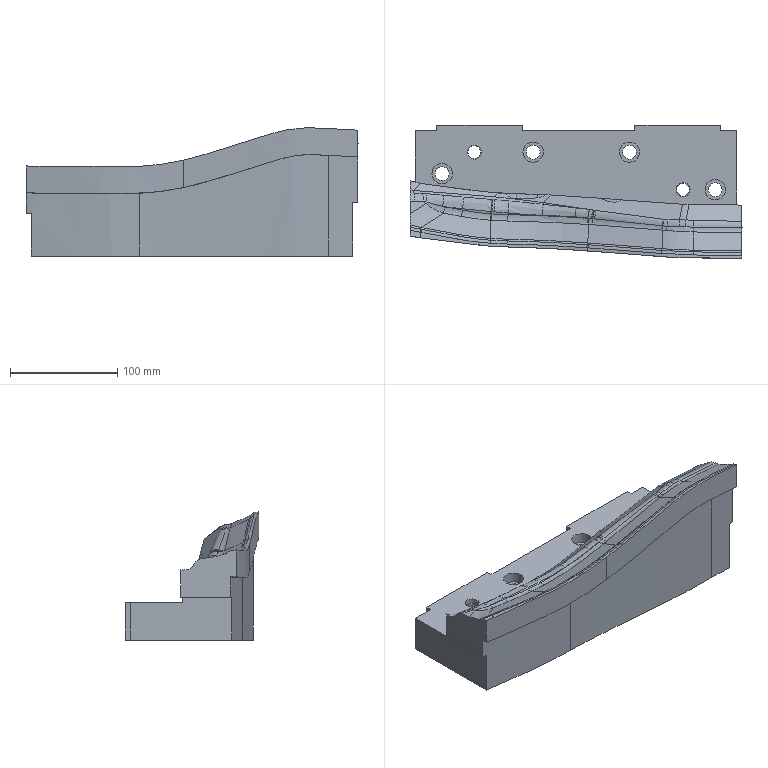Part | NX | features solid 2 | 1 solid | 139 faces | box 310.044 x 124.51 x 119.836 mm | volume 1866888 mm3 | spline 54 | cylinder 53 | plane 32 | commonest cylinder face diameters 20 x9 13 x6 12 x4 19 x4 20.001 x4 10 x3